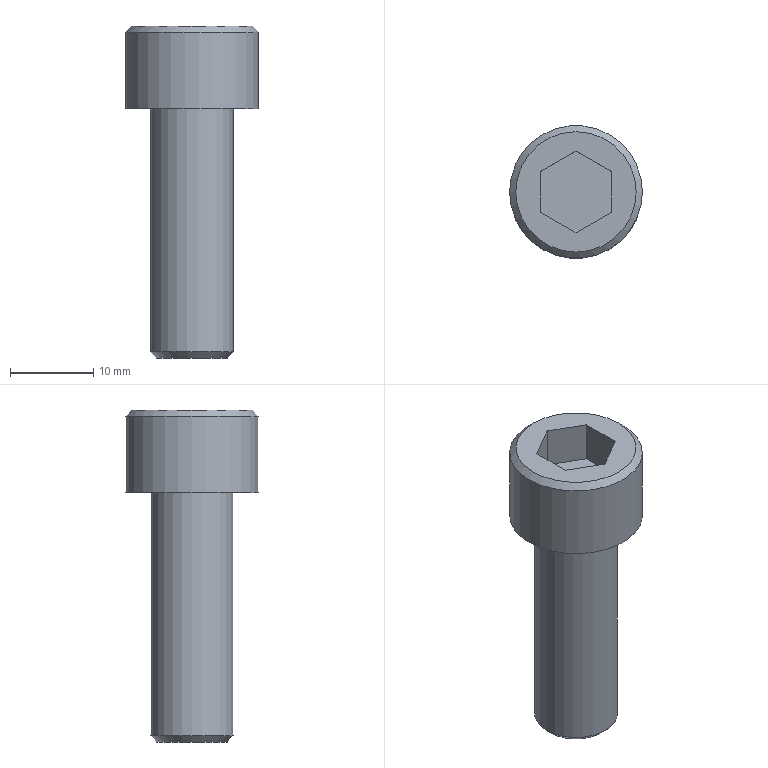Part | STEP file | M10.00-30.00 | 1 solid | 14 faces | box 16 x 16 x 40 mm | volume 4032 mm3 | plane 10 | cylinder 2 | cone 2 | commonest cylinder face diameters 10 x1 16 x1